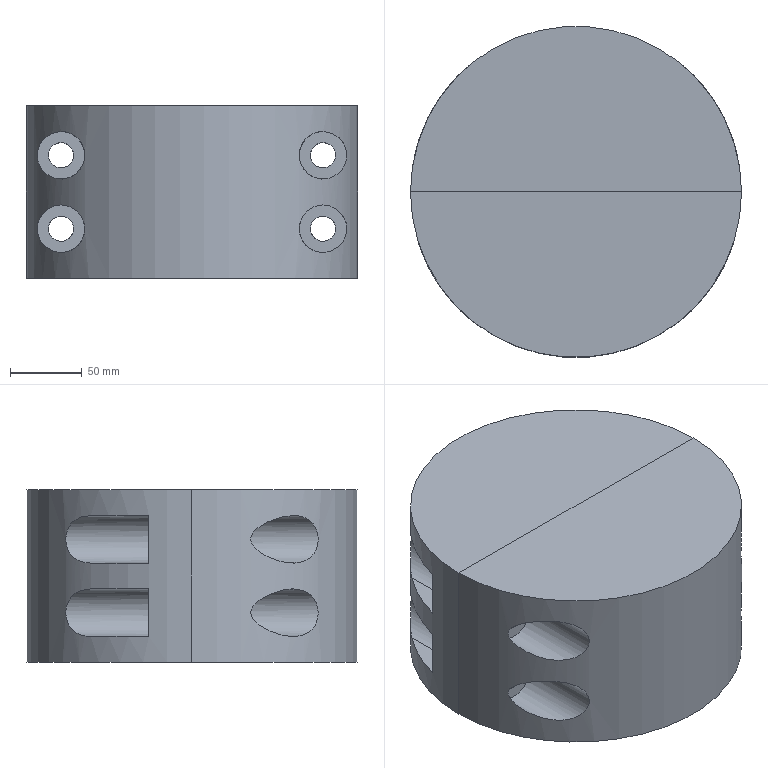NC program | NX | posted with a generic post | part box 230 x 230 x 120 mm
Lines 7936 to 7964 of 7964:
(DRILLING , TOOL : ZXZ)
N15870 T02 M6
N15872 G54
N15874 G17 G0 G90 X-91. Y-25.5 S3500 M3
N15876 G43 Z30. H2
N15878 G94 G81 G98 Z-86. F250. R-82.
N15880 Y25.5
N15882 X91.
N15884 Y-25.5
N15886 G80
N15888 G0 X91. Y-25.5 Z30.
N15890 M5
(DRILLING_COPY , TOOL : 21.5ZT)
N15892 T03 M6
N15894 G54
N15896 G17 G0 G90 X-91. Y-25.5 S500 M3
N15898 G43 Z30. H3
N15900 G94 G83 G98 Z-125.959 F80. Q3. R-82.
N15902 Y25.5
N15904 X91.
N15906 Y-25.5
N15908 G80
N15910 G0 X91. Y-25.5 Z30.
N15912 M5
N15914 M2